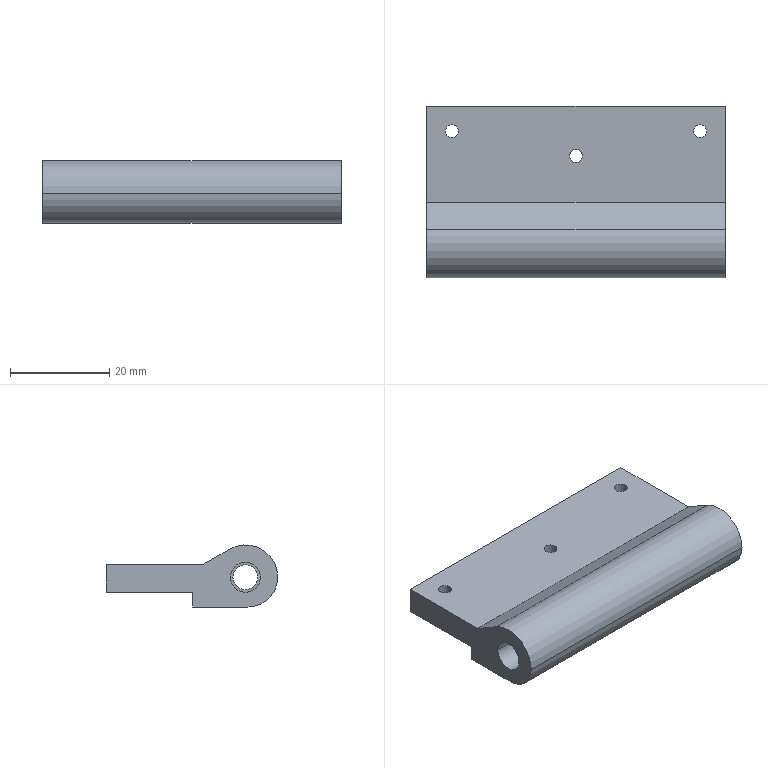NC program | NX | posted with a generic post | part box 60 x 34.5 x 12.5 mm
Whole program:
N10 G17 G21 G94 G90
(HOLE_MILLING_COPY , TOOL : D4)
N12 T04 M6
N14 G54
N16 G17 G0 G90 X-28. Y-6. B0. C0. S9500 M3
N18 G43 Z30. H4
N20 Z0.5
N22 G94 G3 X-27.545 Y-6.455 R0.455 F1250.
N24 X-27.09 Y-6. R0.455
N26 X-27.09 Y-6. Z0.25 I-0.91 J0.
N28 X-27.09 Y-6. Z0. I-0.91 J0.
N30 X-27.09 Y-6. Z-0.25 I-0.91 J0.
N32 X-27.09 Y-6. Z-0.5 I-0.91 J0.
N34 X-27.09 Y-6. Z-0.75 I-0.91 J0.
N36 X-27.09 Y-6. Z-1. I-0.91 J0.
N38 X-27.09 Y-6. Z-1.25 I-0.91 J0.
N40 X-27.09 Y-6. Z-1.5 I-0.91 J0.
N42 X-27.09 Y-6. Z-1.75 I-0.91 J0.
N44 X-27.09 Y-6. Z-2. I-0.91 J0.
N46 X-27.09 Y-6. Z-2.25 I-0.91 J0.
N48 X-27.09 Y-6. Z-2.5 I-0.91 J0.
N50 X-27.09 Y-6. Z-2.75 I-0.91 J0.
N52 X-27.09 Y-6. Z-3. I-0.91 J0.
N54 X-27.09 Y-6. Z-3.25 I-0.91 J0.
N56 X-27.09 Y-6. Z-3.5 I-0.91 J0.
N58 X-27.09 Y-6. Z-3.75 I-0.91 J0.
N60 X-27.09 Y-6. Z-4. I-0.91 J0.
N62 X-27.09 Y-6. Z-4.25 I-0.91 J0.
N64 X-27.09 Y-6. Z-4.5 I-0.91 J0.
N66 X-27.09 Y-6. Z-4.75 I-0.91 J0.
N68 X-27.09 Y-6. Z-5. I-0.91 J0.
N70 X-27.09 Y-6. Z-5.25 I-0.91 J0.
N72 X-27.09 Y-6. Z-5.5 I-0.91 J0.
N74 X-27.09 Y-6. Z-5.75 I-0.91 J0.
N76 X-27.09 Y-6. Z-6. I-0.91 J0.
N78 X-27.09 Y-6. Z-6.25 I-0.91 J0.
N80 X-27.09 Y-6. Z-6.5 I-0.91 J0.
N82 X-27.09 Y-6. Z-6.75 I-0.91 J0.
N84 X-27.09 Y-6. Z-7. I-0.91 J0.
N86 X-27.09 Y-6. Z-7.25 I-0.91 J0.
N88 X-27.09 Y-6. Z-7.5 I-0.91 J0.
N90 X-27.09 Y-6. Z-7.75 I-0.91 J0.
N92 X-27.09 Y-6. Z-8. I-0.91 J0.
N94 X-27.09 Y-6. Z-8.25 I-0.91 J0.
N96 X-27.09 Y-6. Z-8.5 I-0.91 J0.
N98 X-27.09 Y-6. Z-8.75 I-0.91 J0.
N100 X-27.09 Y-6. Z-9. I-0.91 J0.
N102 X-27.09 Y-6. Z-9.25 I-0.91 J0.
N104 X-27.09 Y-6. Z-9.5 I-0.91 J0.
N106 X-27.09 Y-6. Z-9.75 I-0.91 J0.
N108 X-27.719 Y-5.135 Z-9.8 R0.91
N110 X-28.865 Y-5.719 R0.91
N112 X-27.719 Y-5.135 R-0.91
N114 X-28.292 Y-5.427 R0.455
N116 X-28. Y-6. R0.455
N118 G0 Z30.
N120 M5
(ZLEVEL_PROFILE_1_COPY_1_COPY_COPY_COPY_1_COPY_COPY_COPY_COPY_1_COPY , TOOL : D)
N122 T07 M6
N124 G54
N126 G17 G0 G90 X-27.758 Y-5.184 B0. C0. S9500 M3
N128 G43 Z30. H7
N130 Z0.
N132 G94 G1 Z-1. F1000.
N134 X-27.48 Y-4.249
N136 G3 X-28. Y-3.949 R0.6
N138 X-30.051 Y-6. R2.051
N140 X-28. Y-3.949 R-2.051
N142 X-28.52 Y-4.249 R0.6
N144 G1 X-28.242 Y-5.184
N146 Z0.
N148 G0 Z30.
N150 M5
(CUTTERCOMP4_COPY , TOOL : D4)
N152 T04 M6
N154 G54
N156 G17 G0 G90 X-28. Y-6. B0. C0. S9500 M3
N158 G43 Z30. H4
N160 Z0.5
N162 G41 G94 G1 X-27.997 Y-6.1 F1000. D4
N164 G3 X-27.04 Y-6. R0.484
N166 X-27.04 Y-6. Z-1.5 I-0.96 J0.
N168 X-27.04 Y-6. Z-3.5 I-0.96 J0.
N170 X-27.04 Y-6. Z-5.5 I-0.96 J0.
N172 X-27.04 Y-6. Z-7.5 I-0.96 J0.
N174 X-27.04 Y-6. Z-9.5 I-0.96 J0.
N176 X-27.436 Y-5.223 Z-9.8 R0.96
N178 X-28.777 Y-5.436 R0.96
N180 X-27.436 Y-5.223 R-0.96
N182 X-28.079 Y-5.939 R0.484
N184 G40
N186 G1 X-28. Y-6.
N188 G0 Z30.
N190 M5
N192 M2